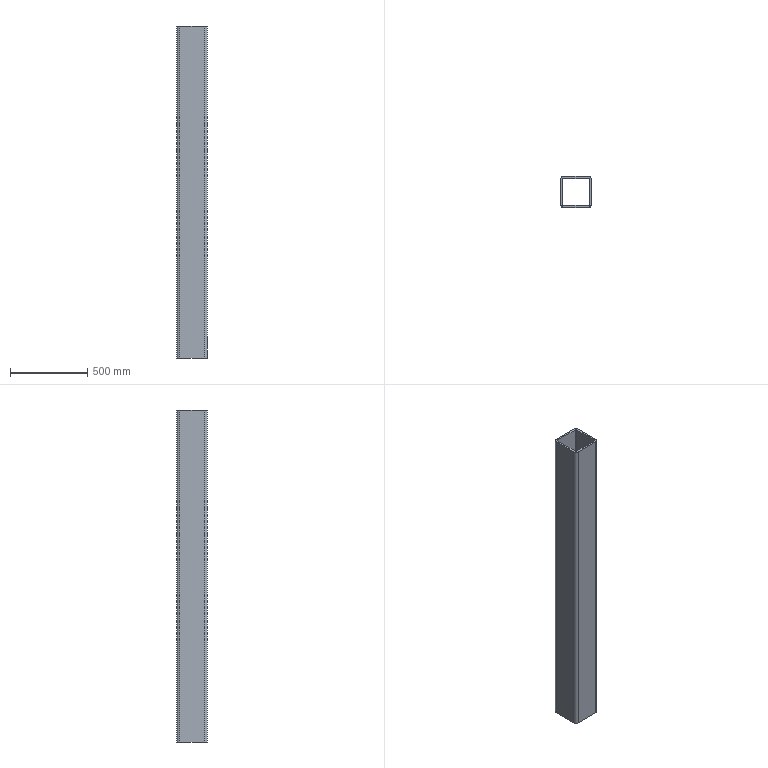Part | SolidWorks | features Extrusion 1, Fillet 1, ICE 1 | 1 solid | 23 faces | box 200 x 200 x 2150 mm | volume 18654812 mm3 | plane 12 | cylinder 11 | commonest cylinder face diameters 16 x4 40 x4 20 x2 80 x1
STEP:
#1=CARTESIAN_POINT('',(80.,-100.,2150.));
#2=VERTEX_POINT('',#1);
#3=CARTESIAN_POINT('',(100.,-80.,2150.));
#4=VERTEX_POINT('',#3);
#5=CARTESIAN_POINT('',(80.,-80.,2150.));
#6=DIRECTION('',(0.,0.,1.));
#7=DIRECTION('',(1.,0.,0.));
#8=AXIS2_PLACEMENT_3D('',#5,#6,#7);
#9=CIRCLE('',#8,20.);
#10=EDGE_CURVE('',#2,#4,#9,.T.);
#11=ORIENTED_EDGE('',*,*,#10,.T.);
#12=CARTESIAN_POINT('',(100.,80.,2150.));
#13=VERTEX_POINT('',#12);
#14=CARTESIAN_POINT('',(100.,80.,2150.));
#15=DIRECTION('',(0.,1.,0.));
#16=VECTOR('',#15,1000.);
#17=LINE('',#14,#16);
#18=EDGE_CURVE('',#4,#13,#17,.T.);
#19=ORIENTED_EDGE('',*,*,#18,.T.);
#20=CARTESIAN_POINT('',(80.,100.,2150.));
#21=VERTEX_POINT('',#20);
#22=CARTESIAN_POINT('',(80.,80.,2150.));
#23=DIRECTION('',(0.,0.,1.));
#24=DIRECTION('',(1.,0.,0.));
#25=AXIS2_PLACEMENT_3D('',#22,#23,#24);
#26=CIRCLE('',#25,20.);
#27=EDGE_CURVE('',#13,#21,#26,.T.);
#28=ORIENTED_EDGE('',*,*,#27,.T.);
#29=CARTESIAN_POINT('',(-80.,100.,2150.));
#30=VERTEX_POINT('',#29);
#31=CARTESIAN_POINT('',(-80.,100.,2150.));
#32=DIRECTION('',(-1.,0.,0.));
#33=VECTOR('',#32,1000.);
#34=LINE('',#31,#33);
#35=EDGE_CURVE('',#21,#30,#34,.T.);
#36=ORIENTED_EDGE('',*,*,#35,.T.);
#37=CARTESIAN_POINT('',(-100.,80.,2150.));
#38=VERTEX_POINT('',#37);
#39=CARTESIAN_POINT('',(-80.,80.,2150.));
#40=DIRECTION('',(0.,0.,1.));
#41=DIRECTION('',(-1.,0.,0.));
#42=AXIS2_PLACEMENT_3D('',#39,#40,#41);
#43=CIRCLE('',#42,20.);
#44=EDGE_CURVE('',#30,#38,#43,.T.);
#45=ORIENTED_EDGE('',*,*,#44,.T.);
#46=CARTESIAN_POINT('',(-100.,-80.,2150.));
#47=VERTEX_POINT('',#46);
#48=CARTESIAN_POINT('',(-100.,80.,2150.));
#49=DIRECTION('',(0.,-1.,0.));
#50=VECTOR('',#49,1000.);
#51=LINE('',#48,#50);
#52=EDGE_CURVE('',#38,#47,#51,.T.);
#53=ORIENTED_EDGE('',*,*,#52,.T.);
#54=CARTESIAN_POINT('',(-80.,-100.,2150.));
#55=VERTEX_POINT('',#54);
#56=CARTESIAN_POINT('',(-80.,-80.,2150.));
#57=DIRECTION('',(0.,0.,1.));
#58=DIRECTION('',(-1.,0.,0.));
#59=AXIS2_PLACEMENT_3D('',#56,#57,#58);
#60=CIRCLE('',#59,20.);
#61=EDGE_CURVE('',#47,#55,#60,.T.);
#62=ORIENTED_EDGE('',*,*,#61,.T.);
#63=CARTESIAN_POINT('',(-80.,-100.,2150.));
#64=DIRECTION('',(1.,0.,0.));
#65=VECTOR('',#64,1000.);
#66=LINE('',#63,#65);
#67=EDGE_CURVE('',#55,#2,#66,.T.);
#68=ORIENTED_EDGE('',*,*,#67,.T.);
#69=EDGE_LOOP('',(#11,#19,#28,#36,#45,#53,#62,#68));
#70=FACE_OUTER_BOUND('',#69,.T.);
#71=CARTESIAN_POINT('',(-88.,80.,2150.));
#72=VERTEX_POINT('',#71);
#73=CARTESIAN_POINT('',(-88.,-80.,2150.));
#74=VERTEX_POINT('',#73);
#75=CARTESIAN_POINT('',(-88.,80.,2150.));
#76=DIRECTION('',(0.,-1.,0.));
#77=VECTOR('',#76,1000.);
#78=LINE('',#75,#77);
#79=EDGE_CURVE('',#72,#74,#78,.T.);
#80=ORIENTED_EDGE('',*,*,#79,.F.);
#81=CARTESIAN_POINT('',(-80.,88.,2150.));
#82=VERTEX_POINT('',#81);
#83=CARTESIAN_POINT('',(-80.,80.,2150.));
#84=DIRECTION('',(0.,0.,1.));
#85=DIRECTION('',(-1.,0.,0.));
#86=AXIS2_PLACEMENT_3D('',#83,#84,#85);
#87=CIRCLE('',#86,8.);
#88=EDGE_CURVE('',#82,#72,#87,.T.);
#89=ORIENTED_EDGE('',*,*,#88,.F.);
#90=CARTESIAN_POINT('',(80.,88.,2150.));
#91=VERTEX_POINT('',#90);
#92=CARTESIAN_POINT('',(-80.,88.,2150.));
#93=DIRECTION('',(-1.,0.,0.));
#94=VECTOR('',#93,1000.);
#95=LINE('',#92,#94);
#96=EDGE_CURVE('',#91,#82,#95,.T.);
#97=ORIENTED_EDGE('',*,*,#96,.F.);
#98=CARTESIAN_POINT('',(88.,80.,2150.));
#99=VERTEX_POINT('',#98);
#100=CARTESIAN_POINT('',(80.,80.,2150.));
#101=DIRECTION('',(0.,0.,1.));
#102=DIRECTION('',(1.,0.,0.));
#103=AXIS2_PLACEMENT_3D('',#100,#101,#102);
#104=CIRCLE('',#103,8.);
#105=EDGE_CURVE('',#99,#91,#104,.T.);
#106=ORIENTED_EDGE('',*,*,#105,.F.);
#107=CARTESIAN_POINT('',(88.,-80.,2150.));
#108=VERTEX_POINT('',#107);
#109=CARTESIAN_POINT('',(88.,80.,2150.));
#110=DIRECTION('',(0.,1.,0.));
#111=VECTOR('',#110,1000.);
#112=LINE('',#109,#111);
#113=EDGE_CURVE('',#108,#99,#112,.T.);
#114=ORIENTED_EDGE('',*,*,#113,.F.);
#115=CARTESIAN_POINT('',(80.,-88.,2150.));
#116=VERTEX_POINT('',#115);
#117=CARTESIAN_POINT('',(80.,-80.,2150.));
#118=DIRECTION('',(0.,0.,1.));
#119=DIRECTION('',(1.,0.,0.));
#120=AXIS2_PLACEMENT_3D('',#117,#118,#119);
#121=CIRCLE('',#120,8.);
#122=EDGE_CURVE('',#116,#108,#121,.T.);
#123=ORIENTED_EDGE('',*,*,#122,.F.);
#124=CARTESIAN_POINT('',(-80.,-88.,2150.));
#125=VERTEX_POINT('',#124);
#126=CARTESIAN_POINT('',(-80.,-88.,2150.));
#127=DIRECTION('',(1.,0.,0.));
#128=VECTOR('',#127,1000.);
#129=LINE('',#126,#128);
#130=EDGE_CURVE('',#125,#116,#129,.T.);
#131=ORIENTED_EDGE('',*,*,#130,.F.);
#132=CARTESIAN_POINT('',(-80.,-80.,2150.));
#133=DIRECTION('',(0.,0.,1.));
#134=DIRECTION('',(-1.,0.,0.));
#135=AXIS2_PLACEMENT_3D('',#132,#133,#134);
#136=CIRCLE('',#135,8.);
#137=EDGE_CURVE('',#74,#125,#136,.T.);
#138=ORIENTED_EDGE('',*,*,#137,.F.);
#139=EDGE_LOOP('',(#80,#89,#97,#106,#114,#123,#131,#138));
#140=FACE_BOUND('',#139,.T.);
#141=CARTESIAN_POINT('',(80.,-80.,2150.));
#142=DIRECTION('',(0.,0.,1.));
#143=DIRECTION('',(1.,0.,0.));
#144=AXIS2_PLACEMENT_3D('',#141,#142,#143);
#145=PLANE('',#144);
#146=ADVANCED_FACE('',(#70,#140),#145,.T.);
#147=CARTESIAN_POINT('',(88.,-80.,0.));
#148=VERTEX_POINT('',#147);
#149=CARTESIAN_POINT('',(88.,-50.,0.));
#150=VERTEX_POINT('',#149);
#151=CARTESIAN_POINT('',(88.,80.,0.));
#152=DIRECTION('',(0.,1.,0.));
#153=VECTOR('',#152,1000.);
#154=LINE('',#151,#153);
#155=EDGE_CURVE('',#148,#150,#154,.T.);
#156=ORIENTED_EDGE('',*,*,#155,.T.);
#157=CARTESIAN_POINT('',(100.,-50.,0.));
#158=VERTEX_POINT('',#157);
#159=CARTESIAN_POINT('',(80.,-50.,0.));
#160=DIRECTION('',(1.,0.,0.));
#161=VECTOR('',#160,1000.);
#162=LINE('',#159,#161);
#163=EDGE_CURVE('',#150,#158,#162,.T.);
#164=ORIENTED_EDGE('',*,*,#163,.T.);
#165=CARTESIAN_POINT('',(100.,-80.,0.));
#166=VERTEX_POINT('',#165);
#167=CARTESIAN_POINT('',(100.,80.,0.));
#168=DIRECTION('',(0.,1.,0.));
#169=VECTOR('',#168,1000.);
#170=LINE('',#167,#169);
#171=EDGE_CURVE('',#166,#158,#170,.T.);
#172=ORIENTED_EDGE('',*,*,#171,.F.);
#173=CARTESIAN_POINT('',(80.,-100.,0.));
#174=VERTEX_POINT('',#173);
#175=CARTESIAN_POINT('',(80.,-80.,0.));
#176=DIRECTION('',(0.,0.,1.));
#177=DIRECTION('',(1.,0.,0.));
#178=AXIS2_PLACEMENT_3D('',#175,#176,#177);
#179=CIRCLE('',#178,20.);
#180=EDGE_CURVE('',#174,#166,#179,.T.);
#181=ORIENTED_EDGE('',*,*,#180,.F.);
#182=CARTESIAN_POINT('',(-80.,-100.,0.));
#183=VERTEX_POINT('',#182);
#184=CARTESIAN_POINT('',(-80.,-100.,0.));
#185=DIRECTION('',(1.,0.,0.));
#186=VECTOR('',#185,1000.);
#187=LINE('',#184,#186);
#188=EDGE_CURVE('',#183,#174,#187,.T.);
#189=ORIENTED_EDGE('',*,*,#188,.F.);
#190=CARTESIAN_POINT('',(-100.,-80.,0.));
#191=VERTEX_POINT('',#190);
#192=CARTESIAN_POINT('',(-80.,-80.,0.));
#193=DIRECTION('',(0.,0.,1.));
#194=DIRECTION('',(-1.,0.,0.));
#195=AXIS2_PLACEMENT_3D('',#192,#193,#194);
#196=CIRCLE('',#195,20.);
#197=EDGE_CURVE('',#191,#183,#196,.T.);
#198=ORIENTED_EDGE('',*,*,#197,.F.);
#199=CARTESIAN_POINT('',(-100.,80.,0.));
#200=VERTEX_POINT('',#199);
#201=CARTESIAN_POINT('',(-100.,80.,0.));
#202=DIRECTION('',(0.,-1.,0.));
#203=VECTOR('',#202,1000.);
#204=LINE('',#201,#203);
#205=EDGE_CURVE('',#200,#191,#204,.T.);
#206=ORIENTED_EDGE('',*,*,#205,.F.);
#207=CARTESIAN_POINT('',(-80.,100.,0.));
#208=VERTEX_POINT('',#207);
#209=CARTESIAN_POINT('',(-80.,80.,0.));
#210=DIRECTION('',(0.,0.,1.));
#211=DIRECTION('',(-1.,0.,0.));
#212=AXIS2_PLACEMENT_3D('',#209,#210,#211);
#213=CIRCLE('',#212,20.);
#214=EDGE_CURVE('',#208,#200,#213,.T.);
#215=ORIENTED_EDGE('',*,*,#214,.F.);
#216=CARTESIAN_POINT('',(80.,100.,0.));
#217=VERTEX_POINT('',#216);
#218=CARTESIAN_POINT('',(-80.,100.,0.));
#219=DIRECTION('',(-1.,0.,0.));
#220=VECTOR('',#219,1000.);
#221=LINE('',#218,#220);
#222=EDGE_CURVE('',#217,#208,#221,.T.);
#223=ORIENTED_EDGE('',*,*,#222,.F.);
#224=CARTESIAN_POINT('',(100.,80.,0.));
#225=VERTEX_POINT('',#224);
#226=CARTESIAN_POINT('',(80.,80.,0.));
#227=DIRECTION('',(0.,0.,1.));
#228=DIRECTION('',(1.,0.,0.));
#229=AXIS2_PLACEMENT_3D('',#226,#227,#228);
#230=CIRCLE('',#229,20.);
#231=EDGE_CURVE('',#225,#217,#230,.T.);
#232=ORIENTED_EDGE('',*,*,#231,.F.);
#233=CARTESIAN_POINT('',(100.,50.,0.));
#234=VERTEX_POINT('',#233);
#235=CARTESIAN_POINT('',(100.,80.,0.));
#236=DIRECTION('',(0.,1.,0.));
#237=VECTOR('',#236,1000.);
#238=LINE('',#235,#237);
#239=EDGE_CURVE('',#234,#225,#238,.T.);
#240=ORIENTED_EDGE('',*,*,#239,.F.);
#241=CARTESIAN_POINT('',(88.,50.,0.));
#242=VERTEX_POINT('',#241);
#243=CARTESIAN_POINT('',(80.,50.,0.));
#244=DIRECTION('',(-1.,0.,0.));
#245=VECTOR('',#244,1000.);
#246=LINE('',#243,#245);
#247=EDGE_CURVE('',#234,#242,#246,.T.);
#248=ORIENTED_EDGE('',*,*,#247,.T.);
#249=CARTESIAN_POINT('',(88.,80.,0.));
#250=VERTEX_POINT('',#249);
#251=CARTESIAN_POINT('',(88.,80.,0.));
#252=DIRECTION('',(0.,1.,0.));
#253=VECTOR('',#252,1000.);
#254=LINE('',#251,#253);
#255=EDGE_CURVE('',#242,#250,#254,.T.);
#256=ORIENTED_EDGE('',*,*,#255,.T.);
#257=CARTESIAN_POINT('',(80.,88.,0.));
#258=VERTEX_POINT('',#257);
#259=CARTESIAN_POINT('',(80.,80.,0.));
#260=DIRECTION('',(0.,0.,1.));
#261=DIRECTION('',(1.,0.,0.));
#262=AXIS2_PLACEMENT_3D('',#259,#260,#261);
#263=CIRCLE('',#262,8.);
#264=EDGE_CURVE('',#250,#258,#263,.T.);
#265=ORIENTED_EDGE('',*,*,#264,.T.);
#266=CARTESIAN_POINT('',(-80.,88.,0.));
#267=VERTEX_POINT('',#266);
#268=CARTESIAN_POINT('',(-80.,88.,0.));
#269=DIRECTION('',(-1.,0.,0.));
#270=VECTOR('',#269,1000.);
#271=LINE('',#268,#270);
#272=EDGE_CURVE('',#258,#267,#271,.T.);
#273=ORIENTED_EDGE('',*,*,#272,.T.);
#274=CARTESIAN_POINT('',(-88.,80.,0.));
#275=VERTEX_POINT('',#274);
#276=CARTESIAN_POINT('',(-80.,80.,0.));
#277=DIRECTION('',(0.,0.,1.));
#278=DIRECTION('',(-1.,0.,0.));
#279=AXIS2_PLACEMENT_3D('',#276,#277,#278);
#280=CIRCLE('',#279,8.);
#281=EDGE_CURVE('',#267,#275,#280,.T.);
#282=ORIENTED_EDGE('',*,*,#281,.T.);
#283=CARTESIAN_POINT('',(-88.,-80.,0.));
#284=VERTEX_POINT('',#283);
#285=CARTESIAN_POINT('',(-88.,80.,0.));
#286=DIRECTION('',(0.,-1.,0.));
#287=VECTOR('',#286,1000.);
#288=LINE('',#285,#287);
#289=EDGE_CURVE('',#275,#284,#288,.T.);
#290=ORIENTED_EDGE('',*,*,#289,.T.);
#291=CARTESIAN_POINT('',(-80.,-88.,0.));
#292=VERTEX_POINT('',#291);
#293=CARTESIAN_POINT('',(-80.,-80.,0.));
#294=DIRECTION('',(0.,0.,1.));
#295=DIRECTION('',(-1.,0.,0.));
#296=AXIS2_PLACEMENT_3D('',#293,#294,#295);
#297=CIRCLE('',#296,8.);
#298=EDGE_CURVE('',#284,#292,#297,.T.);
#299=ORIENTED_EDGE('',*,*,#298,.T.);
#300=CARTESIAN_POINT('',(80.,-88.,0.));
#301=VERTEX_POINT('',#300);
#302=CARTESIAN_POINT('',(-80.,-88.,0.));
#303=DIRECTION('',(1.,0.,0.));
#304=VECTOR('',#303,1000.);
#305=LINE('',#302,#304);
#306=EDGE_CURVE('',#292,#301,#305,.T.);
#307=ORIENTED_EDGE('',*,*,#306,.T.);
#308=CARTESIAN_POINT('',(80.,-80.,0.));
#309=DIRECTION('',(0.,0.,1.));
#310=DIRECTION('',(1.,0.,0.));
#311=AXIS2_PLACEMENT_3D('',#308,#309,#310);
#312=CIRCLE('',#311,8.);
#313=EDGE_CURVE('',#301,#148,#312,.T.);
#314=ORIENTED_EDGE('',*,*,#313,.T.);
#315=EDGE_LOOP('',(#156,#164,#172,#181,#189,#198,#206,#215,#223,#232,#240,#248,#256,#265,#273,#282,#290,#299,#307,#314));
#316=FACE_OUTER_BOUND('',#315,.T.);
#317=CARTESIAN_POINT('',(80.,-80.,0.));
#318=DIRECTION('',(0.,0.,1.));
#319=DIRECTION('',(1.,0.,0.));
#320=AXIS2_PLACEMENT_3D('',#317,#318,#319);
#321=PLANE('',#320);
#322=ADVANCED_FACE('',(#316),#321,.F.);
#323=ORIENTED_EDGE('',*,*,#180,.T.);
#324=CARTESIAN_POINT('',(100.,-80.,2150.));
#325=DIRECTION('',(0.,0.,-1.));
#326=VECTOR('',#325,1000.);
#327=LINE('',#324,#326);
#328=EDGE_CURVE('',#4,#166,#327,.T.);
#329=ORIENTED_EDGE('',*,*,#328,.F.);
#330=ORIENTED_EDGE('',*,*,#10,.F.);
#331=CARTESIAN_POINT('',(80.,-100.,2150.));
#332=DIRECTION('',(0.,0.,-1.));
#333=VECTOR('',#332,1000.);
#334=LINE('',#331,#333);
#335=EDGE_CURVE('',#2,#174,#334,.T.);
#336=ORIENTED_EDGE('',*,*,#335,.T.);
#337=EDGE_LOOP('',(#323,#329,#330,#336));
#338=FACE_OUTER_BOUND('',#337,.T.);
#339=CARTESIAN_POINT('',(80.,-80.,2150.));
#340=DIRECTION('',(0.,0.,-1.));
#341=DIRECTION('',(-1.,0.,0.));
#342=AXIS2_PLACEMENT_3D('',#339,#340,#341);
#343=CYLINDRICAL_SURFACE('',#342,20.);
#344=ADVANCED_FACE('',(#338),#343,.T.);
#345=ORIENTED_EDGE('',*,*,#171,.T.);
#346=CARTESIAN_POINT('',(100.,-40.,10.));
#347=VERTEX_POINT('',#346);
#348=CARTESIAN_POINT('',(100.,-50.,10.));
#349=DIRECTION('',(1.,0.,0.));
#350=DIRECTION('',(0.,-1.,0.));
#351=AXIS2_PLACEMENT_3D('',#348,#349,#350);
#352=CIRCLE('',#351,10.);
#353=EDGE_CURVE('',#158,#347,#352,.T.);
#354=ORIENTED_EDGE('',*,*,#353,.T.);
#355=CARTESIAN_POINT('',(100.,-40.,100.));
#356=VERTEX_POINT('',#355);
#357=CARTESIAN_POINT('',(100.,-40.,100.));
#358=DIRECTION('',(0.,0.,-1.));
#359=VECTOR('',#358,1000.);
#360=LINE('',#357,#359);
#361=EDGE_CURVE('',#356,#347,#360,.T.);
#362=ORIENTED_EDGE('',*,*,#361,.F.);
#363=CARTESIAN_POINT('',(100.,40.,100.));
#364=VERTEX_POINT('',#363);
#365=CARTESIAN_POINT('',(100.,0.,100.));
#366=DIRECTION('',(1.,0.,0.));
#367=DIRECTION('',(0.,1.,0.));
#368=AXIS2_PLACEMENT_3D('',#365,#366,#367);
#369=CIRCLE('',#368,40.);
#370=EDGE_CURVE('',#364,#356,#369,.T.);
#371=ORIENTED_EDGE('',*,*,#370,.F.);
#372=CARTESIAN_POINT('',(100.,40.,10.));
#373=VERTEX_POINT('',#372);
#374=CARTESIAN_POINT('',(100.,40.,100.));
#375=DIRECTION('',(0.,0.,1.));
#376=VECTOR('',#375,1000.);
#377=LINE('',#374,#376);
#378=EDGE_CURVE('',#373,#364,#377,.T.);
#379=ORIENTED_EDGE('',*,*,#378,.F.);
#380=CARTESIAN_POINT('',(100.,50.,10.));
#381=DIRECTION('',(1.,0.,0.));
#382=DIRECTION('',(0.,-1.,0.));
#383=AXIS2_PLACEMENT_3D('',#380,#381,#382);
#384=CIRCLE('',#383,10.);
#385=EDGE_CURVE('',#373,#234,#384,.T.);
#386=ORIENTED_EDGE('',*,*,#385,.T.);
#387=ORIENTED_EDGE('',*,*,#239,.T.);
#388=CARTESIAN_POINT('',(100.,80.,2150.));
#389=DIRECTION('',(0.,0.,-1.));
#390=VECTOR('',#389,1000.);
#391=LINE('',#388,#390);
#392=EDGE_CURVE('',#13,#225,#391,.T.);
#393=ORIENTED_EDGE('',*,*,#392,.F.);
#394=ORIENTED_EDGE('',*,*,#18,.F.);
#395=ORIENTED_EDGE('',*,*,#328,.T.);
#396=EDGE_LOOP('',(#345,#354,#362,#371,#379,#386,#387,#393,#394,#395));
#397=FACE_OUTER_BOUND('',#396,.T.);
#398=CARTESIAN_POINT('',(100.,80.,2150.));
#399=DIRECTION('',(-1.,0.,0.));
#400=DIRECTION('',(0.,-1.,0.));
#401=AXIS2_PLACEMENT_3D('',#398,#399,#400);
#402=PLANE('',#401);
#403=ADVANCED_FACE('',(#397),#402,.F.);
#404=ORIENTED_EDGE('',*,*,#231,.T.);
#405=CARTESIAN_POINT('',(80.,100.,2150.));
#406=DIRECTION('',(0.,0.,-1.));
#407=VECTOR('',#406,1000.);
#408=LINE('',#405,#407);
#409=EDGE_CURVE('',#21,#217,#408,.T.);
#410=ORIENTED_EDGE('',*,*,#409,.F.);
#411=ORIENTED_EDGE('',*,*,#27,.F.);
#412=ORIENTED_EDGE('',*,*,#392,.T.);
#413=EDGE_LOOP('',(#404,#410,#411,#412));
#414=FACE_OUTER_BOUND('',#413,.T.);
#415=CARTESIAN_POINT('',(80.,80.,2150.));
#416=DIRECTION('',(0.,0.,-1.));
#417=DIRECTION('',(-1.,0.,0.));
#418=AXIS2_PLACEMENT_3D('',#415,#416,#417);
#419=CYLINDRICAL_SURFACE('',#418,20.);
#420=ADVANCED_FACE('',(#414),#419,.T.);
#421=ORIENTED_EDGE('',*,*,#222,.T.);
#422=CARTESIAN_POINT('',(-80.,100.,2150.));
#423=DIRECTION('',(0.,0.,-1.));
#424=VECTOR('',#423,1000.);
#425=LINE('',#422,#424);
#426=EDGE_CURVE('',#30,#208,#425,.T.);
#427=ORIENTED_EDGE('',*,*,#426,.F.);
#428=ORIENTED_EDGE('',*,*,#35,.F.);
#429=ORIENTED_EDGE('',*,*,#409,.T.);
#430=EDGE_LOOP('',(#421,#427,#428,#429));
#431=FACE_OUTER_BOUND('',#430,.T.);
#432=CARTESIAN_POINT('',(-80.,100.,2150.));
#433=DIRECTION('',(0.,-1.,0.));
#434=DIRECTION('',(0.,0.,-1.));
#435=AXIS2_PLACEMENT_3D('',#432,#433,#434);
#436=PLANE('',#435);
#437=ADVANCED_FACE('',(#431),#436,.F.);
#438=ORIENTED_EDGE('',*,*,#214,.T.);
#439=CARTESIAN_POINT('',(-100.,80.,2150.));
#440=DIRECTION('',(0.,0.,-1.));
#441=VECTOR('',#440,1000.);
#442=LINE('',#439,#441);
#443=EDGE_CURVE('',#38,#200,#442,.T.);
#444=ORIENTED_EDGE('',*,*,#443,.F.);
#445=ORIENTED_EDGE('',*,*,#44,.F.);
#446=ORIENTED_EDGE('',*,*,#426,.T.);
#447=EDGE_LOOP('',(#438,#444,#445,#446));
#448=FACE_OUTER_BOUND('',#447,.T.);
#449=CARTESIAN_POINT('',(-80.,80.,2150.));
#450=DIRECTION('',(0.,0.,-1.));
#451=DIRECTION('',(-1.,0.,0.));
#452=AXIS2_PLACEMENT_3D('',#449,#450,#451);
#453=CYLINDRICAL_SURFACE('',#452,20.);
#454=ADVANCED_FACE('',(#448),#453,.T.);
#455=ORIENTED_EDGE('',*,*,#205,.T.);
#456=CARTESIAN_POINT('',(-100.,-80.,2150.));
#457=DIRECTION('',(0.,0.,-1.));
#458=VECTOR('',#457,1000.);
#459=LINE('',#456,#458);
#460=EDGE_CURVE('',#47,#191,#459,.T.);
#461=ORIENTED_EDGE('',*,*,#460,.F.);
#462=ORIENTED_EDGE('',*,*,#52,.F.);
#463=ORIENTED_EDGE('',*,*,#443,.T.);
#464=EDGE_LOOP('',(#455,#461,#462,#463));
#465=FACE_OUTER_BOUND('',#464,.T.);
#466=CARTESIAN_POINT('',(-100.,80.,2150.));
#467=DIRECTION('',(1.,0.,0.));
#468=DIRECTION('',(0.,1.,0.));
#469=AXIS2_PLACEMENT_3D('',#466,#467,#468);
#470=PLANE('',#469);
#471=ADVANCED_FACE('',(#465),#470,.F.);
#472=ORIENTED_EDGE('',*,*,#197,.T.);
#473=CARTESIAN_POINT('',(-80.,-100.,2150.));
#474=DIRECTION('',(0.,0.,-1.));
#475=VECTOR('',#474,1000.);
#476=LINE('',#473,#475);
#477=EDGE_CURVE('',#55,#183,#476,.T.);
#478=ORIENTED_EDGE('',*,*,#477,.F.);
#479=ORIENTED_EDGE('',*,*,#61,.F.);
#480=ORIENTED_EDGE('',*,*,#460,.T.);
#481=EDGE_LOOP('',(#472,#478,#479,#480));
#482=FACE_OUTER_BOUND('',#481,.T.);
#483=CARTESIAN_POINT('',(-80.,-80.,2150.));
#484=DIRECTION('',(0.,0.,-1.));
#485=DIRECTION('',(-1.,0.,0.));
#486=AXIS2_PLACEMENT_3D('',#483,#484,#485);
#487=CYLINDRICAL_SURFACE('',#486,20.);
#488=ADVANCED_FACE('',(#482),#487,.T.);
#489=ORIENTED_EDGE('',*,*,#188,.T.);
#490=ORIENTED_EDGE('',*,*,#335,.F.);
#491=ORIENTED_EDGE('',*,*,#67,.F.);
#492=ORIENTED_EDGE('',*,*,#477,.T.);
#493=EDGE_LOOP('',(#489,#490,#491,#492));
#494=FACE_OUTER_BOUND('',#493,.T.);
#495=CARTESIAN_POINT('',(-80.,-100.,2150.));
#496=DIRECTION('',(0.,1.,0.));
#497=DIRECTION('',(-1.,0.,0.));
#498=AXIS2_PLACEMENT_3D('',#495,#496,#497);
#499=PLANE('',#498);
#500=ADVANCED_FACE('',(#494),#499,.F.);
#501=ORIENTED_EDGE('',*,*,#281,.F.);
#502=CARTESIAN_POINT('',(-80.,88.,2150.));
#503=DIRECTION('',(0.,0.,-1.));
#504=VECTOR('',#503,1000.);
#505=LINE('',#502,#504);
#506=EDGE_CURVE('',#82,#267,#505,.T.);
#507=ORIENTED_EDGE('',*,*,#506,.F.);
#508=ORIENTED_EDGE('',*,*,#88,.T.);
#509=CARTESIAN_POINT('',(-88.,80.,2150.));
#510=DIRECTION('',(0.,0.,-1.));
#511=VECTOR('',#510,1000.);
#512=LINE('',#509,#511);
#513=EDGE_CURVE('',#72,#275,#512,.T.);
#514=ORIENTED_EDGE('',*,*,#513,.T.);
#515=EDGE_LOOP('',(#501,#507,#508,#514));
#516=FACE_OUTER_BOUND('',#515,.T.);
#517=CARTESIAN_POINT('',(-80.,80.,2150.));
#518=DIRECTION('',(0.,0.,-1.));
#519=DIRECTION('',(-1.,0.,0.));
#520=AXIS2_PLACEMENT_3D('',#517,#518,#519);
#521=CYLINDRICAL_SURFACE('',#520,8.);
#522=ADVANCED_FACE('',(#516),#521,.F.);
#523=ORIENTED_EDGE('',*,*,#289,.F.);
#524=ORIENTED_EDGE('',*,*,#513,.F.);
#525=ORIENTED_EDGE('',*,*,#79,.T.);
#526=CARTESIAN_POINT('',(-88.,-80.,2150.));
#527=DIRECTION('',(0.,0.,-1.));
#528=VECTOR('',#527,1000.);
#529=LINE('',#526,#528);
#530=EDGE_CURVE('',#74,#284,#529,.T.);
#531=ORIENTED_EDGE('',*,*,#530,.T.);
#532=EDGE_LOOP('',(#523,#524,#525,#531));
#533=FACE_OUTER_BOUND('',#532,.T.);
#534=CARTESIAN_POINT('',(-88.,80.,2150.));
#535=DIRECTION('',(1.,0.,0.));
#536=DIRECTION('',(0.,1.,0.));
#537=AXIS2_PLACEMENT_3D('',#534,#535,#536);
#538=PLANE('',#537);
#539=ADVANCED_FACE('',(#533),#538,.T.);
#540=ORIENTED_EDGE('',*,*,#298,.F.);
#541=ORIENTED_EDGE('',*,*,#530,.F.);
#542=ORIENTED_EDGE('',*,*,#137,.T.);
#543=CARTESIAN_POINT('',(-80.,-88.,2150.));
#544=DIRECTION('',(0.,0.,-1.));
#545=VECTOR('',#544,1000.);
#546=LINE('',#543,#545);
#547=EDGE_CURVE('',#125,#292,#546,.T.);
#548=ORIENTED_EDGE('',*,*,#547,.T.);
#549=EDGE_LOOP('',(#540,#541,#542,#548));
#550=FACE_OUTER_BOUND('',#549,.T.);
#551=CARTESIAN_POINT('',(-80.,-80.,2150.));
#552=DIRECTION('',(0.,0.,-1.));
#553=DIRECTION('',(-1.,0.,0.));
#554=AXIS2_PLACEMENT_3D('',#551,#552,#553);
#555=CYLINDRICAL_SURFACE('',#554,8.);
#556=ADVANCED_FACE('',(#550),#555,.F.);
#557=ORIENTED_EDGE('',*,*,#306,.F.);
#558=ORIENTED_EDGE('',*,*,#547,.F.);
#559=ORIENTED_EDGE('',*,*,#130,.T.);
#560=CARTESIAN_POINT('',(80.,-88.,2150.));
#561=DIRECTION('',(0.,0.,-1.));
#562=VECTOR('',#561,1000.);
#563=LINE('',#560,#562);
#564=EDGE_CURVE('',#116,#301,#563,.T.);
#565=ORIENTED_EDGE('',*,*,#564,.T.);
#566=EDGE_LOOP('',(#557,#558,#559,#565));
#567=FACE_OUTER_BOUND('',#566,.T.);
#568=CARTESIAN_POINT('',(-80.,-88.,2150.));
#569=DIRECTION('',(0.,1.,0.));
#570=DIRECTION('',(0.,0.,1.));
#571=AXIS2_PLACEMENT_3D('',#568,#569,#570);
#572=PLANE('',#571);
#573=ADVANCED_FACE('',(#567),#572,.T.);
#574=ORIENTED_EDGE('',*,*,#313,.F.);
#575=ORIENTED_EDGE('',*,*,#564,.F.);
#576=ORIENTED_EDGE('',*,*,#122,.T.);
#577=CARTESIAN_POINT('',(88.,-80.,2150.));
#578=DIRECTION('',(0.,0.,-1.));
#579=VECTOR('',#578,1000.);
#580=LINE('',#577,#579);
#581=EDGE_CURVE('',#108,#148,#580,.T.);
#582=ORIENTED_EDGE('',*,*,#581,.T.);
#583=EDGE_LOOP('',(#574,#575,#576,#582));
#584=FACE_OUTER_BOUND('',#583,.T.);
#585=CARTESIAN_POINT('',(80.,-80.,2150.));
#586=DIRECTION('',(0.,0.,-1.));
#587=DIRECTION('',(-1.,0.,0.));
#588=AXIS2_PLACEMENT_3D('',#585,#586,#587);
#589=CYLINDRICAL_SURFACE('',#588,8.);
#590=ADVANCED_FACE('',(#584),#589,.F.);
#591=CARTESIAN_POINT('',(88.,-40.,100.));
#592=VERTEX_POINT('',#591);
#593=CARTESIAN_POINT('',(88.,-40.,10.));
#594=VERTEX_POINT('',#593);
#595=CARTESIAN_POINT('',(88.,-40.,100.));
#596=DIRECTION('',(0.,0.,-1.));
#597=VECTOR('',#596,1000.);
#598=LINE('',#595,#597);
#599=EDGE_CURVE('',#592,#594,#598,.T.);
#600=ORIENTED_EDGE('',*,*,#599,.T.);
#601=CARTESIAN_POINT('',(88.,-50.,10.));
#602=DIRECTION('',(-1.,0.,0.));
#603=DIRECTION('',(0.,0.,1.));
#604=AXIS2_PLACEMENT_3D('',#601,#602,#603);
#605=CIRCLE('',#604,10.);
#606=EDGE_CURVE('',#594,#150,#605,.T.);
#607=ORIENTED_EDGE('',*,*,#606,.T.);
#608=ORIENTED_EDGE('',*,*,#155,.F.);
#609=ORIENTED_EDGE('',*,*,#581,.F.);
#610=ORIENTED_EDGE('',*,*,#113,.T.);
#611=CARTESIAN_POINT('',(88.,80.,2150.));
#612=DIRECTION('',(0.,0.,-1.));
#613=VECTOR('',#612,1000.);
#614=LINE('',#611,#613);
#615=EDGE_CURVE('',#99,#250,#614,.T.);
#616=ORIENTED_EDGE('',*,*,#615,.T.);
#617=ORIENTED_EDGE('',*,*,#255,.F.);
#618=CARTESIAN_POINT('',(88.,40.,10.));
#619=VERTEX_POINT('',#618);
#620=CARTESIAN_POINT('',(88.,50.,10.));
#621=DIRECTION('',(-1.,0.,0.));
#622=DIRECTION('',(0.,0.,1.));
#623=AXIS2_PLACEMENT_3D('',#620,#621,#622);
#624=CIRCLE('',#623,10.);
#625=EDGE_CURVE('',#242,#619,#624,.T.);
#626=ORIENTED_EDGE('',*,*,#625,.T.);
#627=CARTESIAN_POINT('',(88.,40.,100.));
#628=VERTEX_POINT('',#627);
#629=CARTESIAN_POINT('',(88.,40.,2150.));
#630=DIRECTION('',(0.,0.,-1.));
#631=VECTOR('',#630,1000.);
#632=LINE('',#629,#631);
#633=EDGE_CURVE('',#628,#619,#632,.T.);
#634=ORIENTED_EDGE('',*,*,#633,.F.);
#635=CARTESIAN_POINT('',(88.,0.,100.));
#636=DIRECTION('',(1.,0.,0.));
#637=DIRECTION('',(0.,0.,1.));
#638=AXIS2_PLACEMENT_3D('',#635,#636,#637);
#639=CIRCLE('',#638,40.);
#640=EDGE_CURVE('',#628,#592,#639,.T.);
#641=ORIENTED_EDGE('',*,*,#640,.T.);
#642=EDGE_LOOP('',(#600,#607,#608,#609,#610,#616,#617,#626,#634,#641));
#643=FACE_OUTER_BOUND('',#642,.T.);
#644=CARTESIAN_POINT('',(88.,80.,2150.));
#645=DIRECTION('',(-1.,0.,0.));
#646=DIRECTION('',(0.,0.,1.));
#647=AXIS2_PLACEMENT_3D('',#644,#645,#646);
#648=PLANE('',#647);
#649=ADVANCED_FACE('',(#643),#648,.T.);
#650=ORIENTED_EDGE('',*,*,#264,.F.);
#651=ORIENTED_EDGE('',*,*,#615,.F.);
#652=ORIENTED_EDGE('',*,*,#105,.T.);
#653=CARTESIAN_POINT('',(80.,88.,2150.));
#654=DIRECTION('',(0.,0.,-1.));
#655=VECTOR('',#654,1000.);
#656=LINE('',#653,#655);
#657=EDGE_CURVE('',#91,#258,#656,.T.);
#658=ORIENTED_EDGE('',*,*,#657,.T.);
#659=EDGE_LOOP('',(#650,#651,#652,#658));
#660=FACE_OUTER_BOUND('',#659,.T.);
#661=CARTESIAN_POINT('',(80.,80.,2150.));
#662=DIRECTION('',(0.,0.,-1.));
#663=DIRECTION('',(-1.,0.,0.));
#664=AXIS2_PLACEMENT_3D('',#661,#662,#663);
#665=CYLINDRICAL_SURFACE('',#664,8.);
#666=ADVANCED_FACE('',(#660),#665,.F.);
#667=ORIENTED_EDGE('',*,*,#272,.F.);
#668=ORIENTED_EDGE('',*,*,#657,.F.);
#669=ORIENTED_EDGE('',*,*,#96,.T.);
#670=ORIENTED_EDGE('',*,*,#506,.T.);
#671=EDGE_LOOP('',(#667,#668,#669,#670));
#672=FACE_OUTER_BOUND('',#671,.T.);
#673=CARTESIAN_POINT('',(-80.,88.,2150.));
#674=DIRECTION('',(0.,-1.,0.));
#675=DIRECTION('',(0.,0.,-1.));
#676=AXIS2_PLACEMENT_3D('',#673,#674,#675);
#677=PLANE('',#676);
#678=ADVANCED_FACE('',(#672),#677,.T.);
#679=ORIENTED_EDGE('',*,*,#361,.T.);
#680=CARTESIAN_POINT('',(-203.204,-40.,10.));
#681=DIRECTION('',(-1.,0.,0.));
#682=VECTOR('',#681,1000.);
#683=LINE('',#680,#682);
#684=EDGE_CURVE('',#347,#594,#683,.T.);
#685=ORIENTED_EDGE('',*,*,#684,.T.);
#686=ORIENTED_EDGE('',*,*,#599,.F.);
#687=CARTESIAN_POINT('',(-203.204,-40.,100.));
#688=DIRECTION('',(1.,0.,0.));
#689=VECTOR('',#688,1000.);
#690=LINE('',#687,#689);
#691=EDGE_CURVE('',#592,#356,#690,.T.);
#692=ORIENTED_EDGE('',*,*,#691,.T.);
#693=EDGE_LOOP('',(#679,#685,#686,#692));
#694=FACE_OUTER_BOUND('',#693,.T.);
#695=CARTESIAN_POINT('',(-203.204,-40.,100.));
#696=DIRECTION('',(0.,-1.,0.));
#697=DIRECTION('',(0.,0.,-1.));
#698=AXIS2_PLACEMENT_3D('',#695,#696,#697);
#699=PLANE('',#698);
#700=ADVANCED_FACE('',(#694),#699,.F.);
#701=ORIENTED_EDGE('',*,*,#633,.T.);
#702=CARTESIAN_POINT('',(-203.204,40.,10.));
#703=DIRECTION('',(1.,0.,0.));
#704=VECTOR('',#703,1000.);
#705=LINE('',#702,#704);
#706=EDGE_CURVE('',#619,#373,#705,.T.);
#707=ORIENTED_EDGE('',*,*,#706,.T.);
#708=ORIENTED_EDGE('',*,*,#378,.T.);
#709=CARTESIAN_POINT('',(-203.204,40.,100.));
#710=DIRECTION('',(1.,0.,0.));
#711=VECTOR('',#710,1000.);
#712=LINE('',#709,#711);
#713=EDGE_CURVE('',#628,#364,#712,.T.);
#714=ORIENTED_EDGE('',*,*,#713,.F.);
#715=EDGE_LOOP('',(#701,#707,#708,#714));
#716=FACE_OUTER_BOUND('',#715,.T.);
#717=CARTESIAN_POINT('',(-203.204,40.,100.));
#718=DIRECTION('',(0.,1.,0.));
#719=DIRECTION('',(0.,0.,1.));
#720=AXIS2_PLACEMENT_3D('',#717,#718,#719);
#721=PLANE('',#720);
#722=ADVANCED_FACE('',(#716),#721,.F.);
#723=ORIENTED_EDGE('',*,*,#713,.T.);
#724=ORIENTED_EDGE('',*,*,#370,.T.);
#725=ORIENTED_EDGE('',*,*,#691,.F.);
#726=ORIENTED_EDGE('',*,*,#640,.F.);
#727=EDGE_LOOP('',(#723,#724,#725,#726));
#728=FACE_OUTER_BOUND('',#727,.T.);
#729=CARTESIAN_POINT('',(-203.204,0.,100.));
#730=DIRECTION('',(1.,0.,0.));
#731=DIRECTION('',(0.,1.,0.));
#732=AXIS2_PLACEMENT_3D('',#729,#730,#731);
#733=CYLINDRICAL_SURFACE('',#732,40.);
#734=ADVANCED_FACE('',(#728),#733,.F.);
#735=ORIENTED_EDGE('',*,*,#606,.F.);
#736=ORIENTED_EDGE('',*,*,#684,.F.);
#737=ORIENTED_EDGE('',*,*,#353,.F.);
#738=ORIENTED_EDGE('',*,*,#163,.F.);
#739=EDGE_LOOP('',(#735,#736,#737,#738));
#740=FACE_OUTER_BOUND('',#739,.T.);
#741=CARTESIAN_POINT('',(80.,-50.,10.));
#742=DIRECTION('',(1.,0.,0.));
#743=DIRECTION('',(0.,1.,0.));
#744=AXIS2_PLACEMENT_3D('',#741,#742,#743);
#745=CYLINDRICAL_SURFACE('',#744,10.);
#746=ADVANCED_FACE('',(#740),#745,.T.);
#747=ORIENTED_EDGE('',*,*,#385,.F.);
#748=ORIENTED_EDGE('',*,*,#706,.F.);
#749=ORIENTED_EDGE('',*,*,#625,.F.);
#750=ORIENTED_EDGE('',*,*,#247,.F.);
#751=EDGE_LOOP('',(#747,#748,#749,#750));
#752=FACE_OUTER_BOUND('',#751,.T.);
#753=CARTESIAN_POINT('',(80.,50.,10.));
#754=DIRECTION('',(-1.,0.,0.));
#755=DIRECTION('',(0.,-1.,0.));
#756=AXIS2_PLACEMENT_3D('',#753,#754,#755);
#757=CYLINDRICAL_SURFACE('',#756,10.);
#758=ADVANCED_FACE('',(#752),#757,.T.);
#759=CLOSED_SHELL('',(#146,#322,#344,#403,#420,#437,#454,#471,#488,#500,#522,#539,#556,#573,#590,#649,#666,#678,#700,#722,#734,#746,#758));
#760=MANIFOLD_SOLID_BREP('',#759);
#761=CARTESIAN_POINT('',(0.,0.,0.));
#762=DIRECTION('',(0.,0.,1.));
#763=DIRECTION('',(1.,0.,0.));
#764=AXIS2_PLACEMENT_3D('',#761,#762,#763);
#765=(LENGTH_UNIT()NAMED_UNIT(*)SI_UNIT(.MILLI.,.METRE.));
#766=UNCERTAINTY_MEASURE_WITH_UNIT(LENGTH_MEASURE(0.00001),#765,'','');
#767=(NAMED_UNIT(*)PLANE_ANGLE_UNIT()SI_UNIT($,.RADIAN.));
#768=(NAMED_UNIT(*)SI_UNIT($,.STERADIAN.)SOLID_ANGLE_UNIT());
#769=(GEOMETRIC_REPRESENTATION_CONTEXT(3)GLOBAL_UNCERTAINTY_ASSIGNED_CONTEXT((#766))GLOBAL_UNIT_ASSIGNED_CONTEXT((#765,#767,#768))REPRESENTATION_CONTEXT('',''));
#770=ADVANCED_BREP_SHAPE_REPRESENTATION('',(#760,#764),#769);